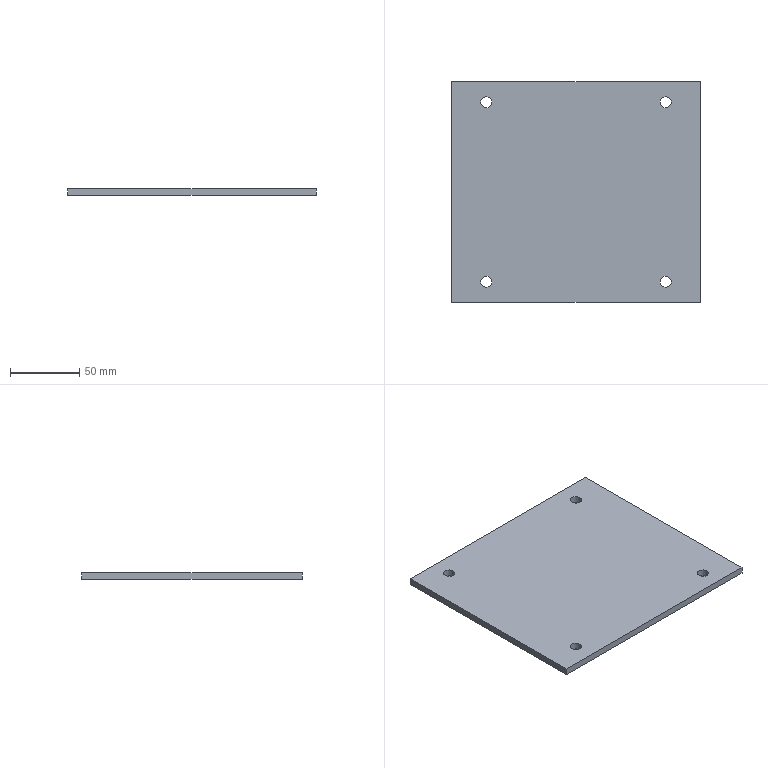Part | SolidWorks | features Extrusion 1, ICE 1 | 1 solid | 14 faces | box 180 x 160 x 5 mm | volume 142995 mm3 | cylinder 8 | plane 6 | commonest cylinder face diameters 8 x8
STEP:
#1=CARTESIAN_POINT('',(-69.,-65.,0.));
#2=VERTEX_POINT('',#1);
#3=CARTESIAN_POINT('',(-61.,-65.,0.));
#4=VERTEX_POINT('',#3);
#5=CARTESIAN_POINT('',(-65.,-65.,0.));
#6=DIRECTION('',(0.,0.,1.));
#7=DIRECTION('',(1.,0.,0.));
#8=AXIS2_PLACEMENT_3D('',#5,#6,#7);
#9=CIRCLE('',#8,4.);
#10=EDGE_CURVE('',#2,#4,#9,.T.);
#11=ORIENTED_EDGE('',*,*,#10,.F.);
#12=CARTESIAN_POINT('',(-69.,-65.,5.));
#13=VERTEX_POINT('',#12);
#14=CARTESIAN_POINT('',(-69.,-65.,0.));
#15=DIRECTION('',(0.,0.,1.));
#16=VECTOR('',#15,1000.);
#17=LINE('',#14,#16);
#18=EDGE_CURVE('',#2,#13,#17,.T.);
#19=ORIENTED_EDGE('',*,*,#18,.T.);
#20=CARTESIAN_POINT('',(-61.,-65.,5.));
#21=VERTEX_POINT('',#20);
#22=CARTESIAN_POINT('',(-65.,-65.,5.));
#23=DIRECTION('',(0.,0.,1.));
#24=DIRECTION('',(1.,0.,0.));
#25=AXIS2_PLACEMENT_3D('',#22,#23,#24);
#26=CIRCLE('',#25,4.);
#27=EDGE_CURVE('',#13,#21,#26,.T.);
#28=ORIENTED_EDGE('',*,*,#27,.T.);
#29=CARTESIAN_POINT('',(-61.,-65.,0.));
#30=DIRECTION('',(0.,0.,1.));
#31=VECTOR('',#30,1000.);
#32=LINE('',#29,#31);
#33=EDGE_CURVE('',#4,#21,#32,.T.);
#34=ORIENTED_EDGE('',*,*,#33,.F.);
#35=EDGE_LOOP('',(#11,#19,#28,#34));
#36=FACE_OUTER_BOUND('',#35,.T.);
#37=CARTESIAN_POINT('',(-65.,-65.,0.));
#38=DIRECTION('',(0.,0.,1.));
#39=DIRECTION('',(1.,0.,0.));
#40=AXIS2_PLACEMENT_3D('',#37,#38,#39);
#41=CYLINDRICAL_SURFACE('',#40,4.);
#42=ADVANCED_FACE('',(#36),#41,.F.);
#43=CARTESIAN_POINT('',(61.,-65.,0.));
#44=VERTEX_POINT('',#43);
#45=CARTESIAN_POINT('',(69.,-65.,0.));
#46=VERTEX_POINT('',#45);
#47=CARTESIAN_POINT('',(65.,-65.,0.));
#48=DIRECTION('',(0.,0.,1.));
#49=DIRECTION('',(1.,0.,0.));
#50=AXIS2_PLACEMENT_3D('',#47,#48,#49);
#51=CIRCLE('',#50,4.);
#52=EDGE_CURVE('',#44,#46,#51,.T.);
#53=ORIENTED_EDGE('',*,*,#52,.F.);
#54=CARTESIAN_POINT('',(61.,-65.,5.));
#55=VERTEX_POINT('',#54);
#56=CARTESIAN_POINT('',(61.,-65.,0.));
#57=DIRECTION('',(0.,0.,1.));
#58=VECTOR('',#57,1000.);
#59=LINE('',#56,#58);
#60=EDGE_CURVE('',#44,#55,#59,.T.);
#61=ORIENTED_EDGE('',*,*,#60,.T.);
#62=CARTESIAN_POINT('',(69.,-65.,5.));
#63=VERTEX_POINT('',#62);
#64=CARTESIAN_POINT('',(65.,-65.,5.));
#65=DIRECTION('',(0.,0.,1.));
#66=DIRECTION('',(1.,0.,0.));
#67=AXIS2_PLACEMENT_3D('',#64,#65,#66);
#68=CIRCLE('',#67,4.);
#69=EDGE_CURVE('',#55,#63,#68,.T.);
#70=ORIENTED_EDGE('',*,*,#69,.T.);
#71=CARTESIAN_POINT('',(69.,-65.,0.));
#72=DIRECTION('',(0.,0.,1.));
#73=VECTOR('',#72,1000.);
#74=LINE('',#71,#73);
#75=EDGE_CURVE('',#46,#63,#74,.T.);
#76=ORIENTED_EDGE('',*,*,#75,.F.);
#77=EDGE_LOOP('',(#53,#61,#70,#76));
#78=FACE_OUTER_BOUND('',#77,.T.);
#79=CARTESIAN_POINT('',(65.,-65.,0.));
#80=DIRECTION('',(0.,0.,1.));
#81=DIRECTION('',(1.,0.,0.));
#82=AXIS2_PLACEMENT_3D('',#79,#80,#81);
#83=CYLINDRICAL_SURFACE('',#82,4.);
#84=ADVANCED_FACE('',(#78),#83,.F.);
#85=CARTESIAN_POINT('',(61.,65.,0.));
#86=VERTEX_POINT('',#85);
#87=CARTESIAN_POINT('',(69.,65.,0.));
#88=VERTEX_POINT('',#87);
#89=CARTESIAN_POINT('',(65.,65.,0.));
#90=DIRECTION('',(0.,0.,1.));
#91=DIRECTION('',(1.,0.,0.));
#92=AXIS2_PLACEMENT_3D('',#89,#90,#91);
#93=CIRCLE('',#92,4.);
#94=EDGE_CURVE('',#86,#88,#93,.T.);
#95=ORIENTED_EDGE('',*,*,#94,.F.);
#96=CARTESIAN_POINT('',(61.,65.,5.));
#97=VERTEX_POINT('',#96);
#98=CARTESIAN_POINT('',(61.,65.,0.));
#99=DIRECTION('',(0.,0.,1.));
#100=VECTOR('',#99,1000.);
#101=LINE('',#98,#100);
#102=EDGE_CURVE('',#86,#97,#101,.T.);
#103=ORIENTED_EDGE('',*,*,#102,.T.);
#104=CARTESIAN_POINT('',(69.,65.,5.));
#105=VERTEX_POINT('',#104);
#106=CARTESIAN_POINT('',(65.,65.,5.));
#107=DIRECTION('',(0.,0.,1.));
#108=DIRECTION('',(1.,0.,0.));
#109=AXIS2_PLACEMENT_3D('',#106,#107,#108);
#110=CIRCLE('',#109,4.);
#111=EDGE_CURVE('',#97,#105,#110,.T.);
#112=ORIENTED_EDGE('',*,*,#111,.T.);
#113=CARTESIAN_POINT('',(69.,65.,0.));
#114=DIRECTION('',(0.,0.,1.));
#115=VECTOR('',#114,1000.);
#116=LINE('',#113,#115);
#117=EDGE_CURVE('',#88,#105,#116,.T.);
#118=ORIENTED_EDGE('',*,*,#117,.F.);
#119=EDGE_LOOP('',(#95,#103,#112,#118));
#120=FACE_OUTER_BOUND('',#119,.T.);
#121=CARTESIAN_POINT('',(65.,65.,0.));
#122=DIRECTION('',(0.,0.,1.));
#123=DIRECTION('',(1.,0.,0.));
#124=AXIS2_PLACEMENT_3D('',#121,#122,#123);
#125=CYLINDRICAL_SURFACE('',#124,4.);
#126=ADVANCED_FACE('',(#120),#125,.F.);
#127=CARTESIAN_POINT('',(-69.,65.,0.));
#128=VERTEX_POINT('',#127);
#129=CARTESIAN_POINT('',(-61.,65.,0.));
#130=VERTEX_POINT('',#129);
#131=CARTESIAN_POINT('',(-65.,65.,0.));
#132=DIRECTION('',(0.,0.,1.));
#133=DIRECTION('',(1.,0.,0.));
#134=AXIS2_PLACEMENT_3D('',#131,#132,#133);
#135=CIRCLE('',#134,4.);
#136=EDGE_CURVE('',#128,#130,#135,.T.);
#137=ORIENTED_EDGE('',*,*,#136,.F.);
#138=CARTESIAN_POINT('',(-69.,65.,5.));
#139=VERTEX_POINT('',#138);
#140=CARTESIAN_POINT('',(-69.,65.,0.));
#141=DIRECTION('',(0.,0.,1.));
#142=VECTOR('',#141,1000.);
#143=LINE('',#140,#142);
#144=EDGE_CURVE('',#128,#139,#143,.T.);
#145=ORIENTED_EDGE('',*,*,#144,.T.);
#146=CARTESIAN_POINT('',(-61.,65.,5.));
#147=VERTEX_POINT('',#146);
#148=CARTESIAN_POINT('',(-65.,65.,5.));
#149=DIRECTION('',(0.,0.,1.));
#150=DIRECTION('',(1.,0.,0.));
#151=AXIS2_PLACEMENT_3D('',#148,#149,#150);
#152=CIRCLE('',#151,4.);
#153=EDGE_CURVE('',#139,#147,#152,.T.);
#154=ORIENTED_EDGE('',*,*,#153,.T.);
#155=CARTESIAN_POINT('',(-61.,65.,0.));
#156=DIRECTION('',(0.,0.,1.));
#157=VECTOR('',#156,1000.);
#158=LINE('',#155,#157);
#159=EDGE_CURVE('',#130,#147,#158,.T.);
#160=ORIENTED_EDGE('',*,*,#159,.F.);
#161=EDGE_LOOP('',(#137,#145,#154,#160));
#162=FACE_OUTER_BOUND('',#161,.T.);
#163=CARTESIAN_POINT('',(-65.,65.,0.));
#164=DIRECTION('',(0.,0.,1.));
#165=DIRECTION('',(1.,0.,0.));
#166=AXIS2_PLACEMENT_3D('',#163,#164,#165);
#167=CYLINDRICAL_SURFACE('',#166,4.);
#168=ADVANCED_FACE('',(#162),#167,.F.);
#169=CARTESIAN_POINT('',(90.,-80.,0.));
#170=VERTEX_POINT('',#169);
#171=CARTESIAN_POINT('',(90.,80.,0.));
#172=VERTEX_POINT('',#171);
#173=CARTESIAN_POINT('',(90.,-80.,0.));
#174=DIRECTION('',(0.,1.,0.));
#175=VECTOR('',#174,1000.);
#176=LINE('',#173,#175);
#177=EDGE_CURVE('',#170,#172,#176,.T.);
#178=ORIENTED_EDGE('',*,*,#177,.T.);
#179=CARTESIAN_POINT('',(90.,80.,5.));
#180=VERTEX_POINT('',#179);
#181=CARTESIAN_POINT('',(90.,80.,5.));
#182=DIRECTION('',(0.,0.,-1.));
#183=VECTOR('',#182,1000.);
#184=LINE('',#181,#183);
#185=EDGE_CURVE('',#180,#172,#184,.T.);
#186=ORIENTED_EDGE('',*,*,#185,.F.);
#187=CARTESIAN_POINT('',(90.,-80.,5.));
#188=VERTEX_POINT('',#187);
#189=CARTESIAN_POINT('',(90.,-80.,5.));
#190=DIRECTION('',(0.,1.,0.));
#191=VECTOR('',#190,1000.);
#192=LINE('',#189,#191);
#193=EDGE_CURVE('',#188,#180,#192,.T.);
#194=ORIENTED_EDGE('',*,*,#193,.F.);
#195=CARTESIAN_POINT('',(90.,-80.,5.));
#196=DIRECTION('',(0.,0.,-1.));
#197=VECTOR('',#196,1000.);
#198=LINE('',#195,#197);
#199=EDGE_CURVE('',#188,#170,#198,.T.);
#200=ORIENTED_EDGE('',*,*,#199,.T.);
#201=EDGE_LOOP('',(#178,#186,#194,#200));
#202=FACE_OUTER_BOUND('',#201,.T.);
#203=CARTESIAN_POINT('',(90.,-80.,5.));
#204=DIRECTION('',(-1.,0.,0.));
#205=DIRECTION('',(0.,0.,1.));
#206=AXIS2_PLACEMENT_3D('',#203,#204,#205);
#207=PLANE('',#206);
#208=ADVANCED_FACE('',(#202),#207,.F.);
#209=CARTESIAN_POINT('',(-90.,80.,0.));
#210=VERTEX_POINT('',#209);
#211=CARTESIAN_POINT('',(-90.,80.,0.));
#212=DIRECTION('',(-1.,0.,0.));
#213=VECTOR('',#212,1000.);
#214=LINE('',#211,#213);
#215=EDGE_CURVE('',#172,#210,#214,.T.);
#216=ORIENTED_EDGE('',*,*,#215,.T.);
#217=CARTESIAN_POINT('',(-90.,80.,5.));
#218=VERTEX_POINT('',#217);
#219=CARTESIAN_POINT('',(-90.,80.,5.));
#220=DIRECTION('',(0.,0.,-1.));
#221=VECTOR('',#220,1000.);
#222=LINE('',#219,#221);
#223=EDGE_CURVE('',#218,#210,#222,.T.);
#224=ORIENTED_EDGE('',*,*,#223,.F.);
#225=CARTESIAN_POINT('',(-90.,80.,5.));
#226=DIRECTION('',(-1.,0.,0.));
#227=VECTOR('',#226,1000.);
#228=LINE('',#225,#227);
#229=EDGE_CURVE('',#180,#218,#228,.T.);
#230=ORIENTED_EDGE('',*,*,#229,.F.);
#231=ORIENTED_EDGE('',*,*,#185,.T.);
#232=EDGE_LOOP('',(#216,#224,#230,#231));
#233=FACE_OUTER_BOUND('',#232,.T.);
#234=CARTESIAN_POINT('',(-90.,80.,5.));
#235=DIRECTION('',(0.,-1.,0.));
#236=DIRECTION('',(0.,0.,-1.));
#237=AXIS2_PLACEMENT_3D('',#234,#235,#236);
#238=PLANE('',#237);
#239=ADVANCED_FACE('',(#233),#238,.F.);
#240=CARTESIAN_POINT('',(-90.,-80.,0.));
#241=VERTEX_POINT('',#240);
#242=CARTESIAN_POINT('',(-90.,-80.,0.));
#243=DIRECTION('',(0.,-1.,0.));
#244=VECTOR('',#243,1000.);
#245=LINE('',#242,#244);
#246=EDGE_CURVE('',#210,#241,#245,.T.);
#247=ORIENTED_EDGE('',*,*,#246,.T.);
#248=CARTESIAN_POINT('',(-90.,-80.,5.));
#249=VERTEX_POINT('',#248);
#250=CARTESIAN_POINT('',(-90.,-80.,5.));
#251=DIRECTION('',(0.,0.,-1.));
#252=VECTOR('',#251,1000.);
#253=LINE('',#250,#252);
#254=EDGE_CURVE('',#249,#241,#253,.T.);
#255=ORIENTED_EDGE('',*,*,#254,.F.);
#256=CARTESIAN_POINT('',(-90.,-80.,5.));
#257=DIRECTION('',(0.,-1.,0.));
#258=VECTOR('',#257,1000.);
#259=LINE('',#256,#258);
#260=EDGE_CURVE('',#218,#249,#259,.T.);
#261=ORIENTED_EDGE('',*,*,#260,.F.);
#262=ORIENTED_EDGE('',*,*,#223,.T.);
#263=EDGE_LOOP('',(#247,#255,#261,#262));
#264=FACE_OUTER_BOUND('',#263,.T.);
#265=CARTESIAN_POINT('',(-90.,-80.,5.));
#266=DIRECTION('',(1.,0.,0.));
#267=DIRECTION('',(0.,0.,-1.));
#268=AXIS2_PLACEMENT_3D('',#265,#266,#267);
#269=PLANE('',#268);
#270=ADVANCED_FACE('',(#264),#269,.F.);
#271=CARTESIAN_POINT('',(-90.,-80.,0.));
#272=DIRECTION('',(1.,0.,0.));
#273=VECTOR('',#272,1000.);
#274=LINE('',#271,#273);
#275=EDGE_CURVE('',#241,#170,#274,.T.);
#276=ORIENTED_EDGE('',*,*,#275,.T.);
#277=ORIENTED_EDGE('',*,*,#199,.F.);
#278=CARTESIAN_POINT('',(-90.,-80.,5.));
#279=DIRECTION('',(1.,0.,0.));
#280=VECTOR('',#279,1000.);
#281=LINE('',#278,#280);
#282=EDGE_CURVE('',#249,#188,#281,.T.);
#283=ORIENTED_EDGE('',*,*,#282,.F.);
#284=ORIENTED_EDGE('',*,*,#254,.T.);
#285=EDGE_LOOP('',(#276,#277,#283,#284));
#286=FACE_OUTER_BOUND('',#285,.T.);
#287=CARTESIAN_POINT('',(-90.,-80.,5.));
#288=DIRECTION('',(0.,1.,0.));
#289=DIRECTION('',(0.,0.,1.));
#290=AXIS2_PLACEMENT_3D('',#287,#288,#289);
#291=PLANE('',#290);
#292=ADVANCED_FACE('',(#286),#291,.F.);
#293=CARTESIAN_POINT('',(-65.,-65.,5.));
#294=DIRECTION('',(0.,0.,1.));
#295=DIRECTION('',(1.,0.,0.));
#296=AXIS2_PLACEMENT_3D('',#293,#294,#295);
#297=CIRCLE('',#296,4.);
#298=EDGE_CURVE('',#21,#13,#297,.T.);
#299=ORIENTED_EDGE('',*,*,#298,.F.);
#300=ORIENTED_EDGE('',*,*,#27,.F.);
#301=EDGE_LOOP('',(#299,#300));
#302=FACE_BOUND('',#301,.T.);
#303=CARTESIAN_POINT('',(65.,-65.,5.));
#304=DIRECTION('',(0.,0.,1.));
#305=DIRECTION('',(1.,0.,0.));
#306=AXIS2_PLACEMENT_3D('',#303,#304,#305);
#307=CIRCLE('',#306,4.);
#308=EDGE_CURVE('',#63,#55,#307,.T.);
#309=ORIENTED_EDGE('',*,*,#308,.F.);
#310=ORIENTED_EDGE('',*,*,#69,.F.);
#311=EDGE_LOOP('',(#309,#310));
#312=FACE_BOUND('',#311,.T.);
#313=CARTESIAN_POINT('',(65.,65.,5.));
#314=DIRECTION('',(0.,0.,1.));
#315=DIRECTION('',(1.,0.,0.));
#316=AXIS2_PLACEMENT_3D('',#313,#314,#315);
#317=CIRCLE('',#316,4.);
#318=EDGE_CURVE('',#105,#97,#317,.T.);
#319=ORIENTED_EDGE('',*,*,#318,.F.);
#320=ORIENTED_EDGE('',*,*,#111,.F.);
#321=EDGE_LOOP('',(#319,#320));
#322=FACE_BOUND('',#321,.T.);
#323=CARTESIAN_POINT('',(-65.,65.,5.));
#324=DIRECTION('',(0.,0.,1.));
#325=DIRECTION('',(1.,0.,0.));
#326=AXIS2_PLACEMENT_3D('',#323,#324,#325);
#327=CIRCLE('',#326,4.);
#328=EDGE_CURVE('',#147,#139,#327,.T.);
#329=ORIENTED_EDGE('',*,*,#328,.F.);
#330=ORIENTED_EDGE('',*,*,#153,.F.);
#331=EDGE_LOOP('',(#329,#330));
#332=FACE_BOUND('',#331,.T.);
#333=ORIENTED_EDGE('',*,*,#193,.T.);
#334=ORIENTED_EDGE('',*,*,#229,.T.);
#335=ORIENTED_EDGE('',*,*,#260,.T.);
#336=ORIENTED_EDGE('',*,*,#282,.T.);
#337=EDGE_LOOP('',(#333,#334,#335,#336));
#338=FACE_OUTER_BOUND('',#337,.T.);
#339=CARTESIAN_POINT('',(0.,0.,5.));
#340=DIRECTION('',(0.,0.,-1.));
#341=DIRECTION('',(-1.,0.,0.));
#342=AXIS2_PLACEMENT_3D('',#339,#340,#341);
#343=PLANE('',#342);
#344=ADVANCED_FACE('',(#302,#312,#322,#332,#338),#343,.F.);
#345=CARTESIAN_POINT('',(-65.,-65.,0.));
#346=DIRECTION('',(0.,0.,1.));
#347=DIRECTION('',(1.,0.,0.));
#348=AXIS2_PLACEMENT_3D('',#345,#346,#347);
#349=CIRCLE('',#348,4.);
#350=EDGE_CURVE('',#4,#2,#349,.T.);
#351=ORIENTED_EDGE('',*,*,#350,.T.);
#352=ORIENTED_EDGE('',*,*,#10,.T.);
#353=EDGE_LOOP('',(#351,#352));
#354=FACE_BOUND('',#353,.T.);
#355=CARTESIAN_POINT('',(65.,-65.,0.));
#356=DIRECTION('',(0.,0.,1.));
#357=DIRECTION('',(1.,0.,0.));
#358=AXIS2_PLACEMENT_3D('',#355,#356,#357);
#359=CIRCLE('',#358,4.);
#360=EDGE_CURVE('',#46,#44,#359,.T.);
#361=ORIENTED_EDGE('',*,*,#360,.T.);
#362=ORIENTED_EDGE('',*,*,#52,.T.);
#363=EDGE_LOOP('',(#361,#362));
#364=FACE_BOUND('',#363,.T.);
#365=CARTESIAN_POINT('',(65.,65.,0.));
#366=DIRECTION('',(0.,0.,1.));
#367=DIRECTION('',(1.,0.,0.));
#368=AXIS2_PLACEMENT_3D('',#365,#366,#367);
#369=CIRCLE('',#368,4.);
#370=EDGE_CURVE('',#88,#86,#369,.T.);
#371=ORIENTED_EDGE('',*,*,#370,.T.);
#372=ORIENTED_EDGE('',*,*,#94,.T.);
#373=EDGE_LOOP('',(#371,#372));
#374=FACE_BOUND('',#373,.T.);
#375=CARTESIAN_POINT('',(-65.,65.,0.));
#376=DIRECTION('',(0.,0.,1.));
#377=DIRECTION('',(1.,0.,0.));
#378=AXIS2_PLACEMENT_3D('',#375,#376,#377);
#379=CIRCLE('',#378,4.);
#380=EDGE_CURVE('',#130,#128,#379,.T.);
#381=ORIENTED_EDGE('',*,*,#380,.T.);
#382=ORIENTED_EDGE('',*,*,#136,.T.);
#383=EDGE_LOOP('',(#381,#382));
#384=FACE_BOUND('',#383,.T.);
#385=ORIENTED_EDGE('',*,*,#177,.F.);
#386=ORIENTED_EDGE('',*,*,#275,.F.);
#387=ORIENTED_EDGE('',*,*,#246,.F.);
#388=ORIENTED_EDGE('',*,*,#215,.F.);
#389=EDGE_LOOP('',(#385,#386,#387,#388));
#390=FACE_OUTER_BOUND('',#389,.T.);
#391=CARTESIAN_POINT('',(0.,0.,0.));
#392=DIRECTION('',(0.,0.,-1.));
#393=DIRECTION('',(-1.,0.,0.));
#394=AXIS2_PLACEMENT_3D('',#391,#392,#393);
#395=PLANE('',#394);
#396=ADVANCED_FACE('',(#354,#364,#374,#384,#390),#395,.T.);
#397=ORIENTED_EDGE('',*,*,#144,.F.);
#398=ORIENTED_EDGE('',*,*,#380,.F.);
#399=ORIENTED_EDGE('',*,*,#159,.T.);
#400=ORIENTED_EDGE('',*,*,#328,.T.);
#401=EDGE_LOOP('',(#397,#398,#399,#400));
#402=FACE_OUTER_BOUND('',#401,.T.);
#403=CARTESIAN_POINT('',(-65.,65.,0.));
#404=DIRECTION('',(0.,0.,1.));
#405=DIRECTION('',(1.,0.,0.));
#406=AXIS2_PLACEMENT_3D('',#403,#404,#405);
#407=CYLINDRICAL_SURFACE('',#406,4.);
#408=ADVANCED_FACE('',(#402),#407,.F.);
#409=ORIENTED_EDGE('',*,*,#102,.F.);
#410=ORIENTED_EDGE('',*,*,#370,.F.);
#411=ORIENTED_EDGE('',*,*,#117,.T.);
#412=ORIENTED_EDGE('',*,*,#318,.T.);
#413=EDGE_LOOP('',(#409,#410,#411,#412));
#414=FACE_OUTER_BOUND('',#413,.T.);
#415=CARTESIAN_POINT('',(65.,65.,0.));
#416=DIRECTION('',(0.,0.,1.));
#417=DIRECTION('',(1.,0.,0.));
#418=AXIS2_PLACEMENT_3D('',#415,#416,#417);
#419=CYLINDRICAL_SURFACE('',#418,4.);
#420=ADVANCED_FACE('',(#414),#419,.F.);
#421=ORIENTED_EDGE('',*,*,#60,.F.);
#422=ORIENTED_EDGE('',*,*,#360,.F.);
#423=ORIENTED_EDGE('',*,*,#75,.T.);
#424=ORIENTED_EDGE('',*,*,#308,.T.);
#425=EDGE_LOOP('',(#421,#422,#423,#424));
#426=FACE_OUTER_BOUND('',#425,.T.);
#427=CARTESIAN_POINT('',(65.,-65.,0.));
#428=DIRECTION('',(0.,0.,1.));
#429=DIRECTION('',(1.,0.,0.));
#430=AXIS2_PLACEMENT_3D('',#427,#428,#429);
#431=CYLINDRICAL_SURFACE('',#430,4.);
#432=ADVANCED_FACE('',(#426),#431,.F.);
#433=ORIENTED_EDGE('',*,*,#18,.F.);
#434=ORIENTED_EDGE('',*,*,#350,.F.);
#435=ORIENTED_EDGE('',*,*,#33,.T.);
#436=ORIENTED_EDGE('',*,*,#298,.T.);
#437=EDGE_LOOP('',(#433,#434,#435,#436));
#438=FACE_OUTER_BOUND('',#437,.T.);
#439=CARTESIAN_POINT('',(-65.,-65.,0.));
#440=DIRECTION('',(0.,0.,1.));
#441=DIRECTION('',(1.,0.,0.));
#442=AXIS2_PLACEMENT_3D('',#439,#440,#441);
#443=CYLINDRICAL_SURFACE('',#442,4.);
#444=ADVANCED_FACE('',(#438),#443,.F.);
#445=CLOSED_SHELL('',(#42,#84,#126,#168,#208,#239,#270,#292,#344,#396,#408,#420,#432,#444));
#446=MANIFOLD_SOLID_BREP('',#445);
#447=CARTESIAN_POINT('',(0.,0.,0.));
#448=DIRECTION('',(0.,0.,1.));
#449=DIRECTION('',(1.,0.,0.));
#450=AXIS2_PLACEMENT_3D('',#447,#448,#449);
#451=(LENGTH_UNIT()NAMED_UNIT(*)SI_UNIT(.MILLI.,.METRE.));
#452=UNCERTAINTY_MEASURE_WITH_UNIT(LENGTH_MEASURE(0.00001),#451,'','');
#453=(NAMED_UNIT(*)PLANE_ANGLE_UNIT()SI_UNIT($,.RADIAN.));
#454=(NAMED_UNIT(*)SI_UNIT($,.STERADIAN.)SOLID_ANGLE_UNIT());
#455=(GEOMETRIC_REPRESENTATION_CONTEXT(3)GLOBAL_UNCERTAINTY_ASSIGNED_CONTEXT((#452))GLOBAL_UNIT_ASSIGNED_CONTEXT((#451,#453,#454))REPRESENTATION_CONTEXT('',''));
#456=ADVANCED_BREP_SHAPE_REPRESENTATION('',(#446,#450),#455);